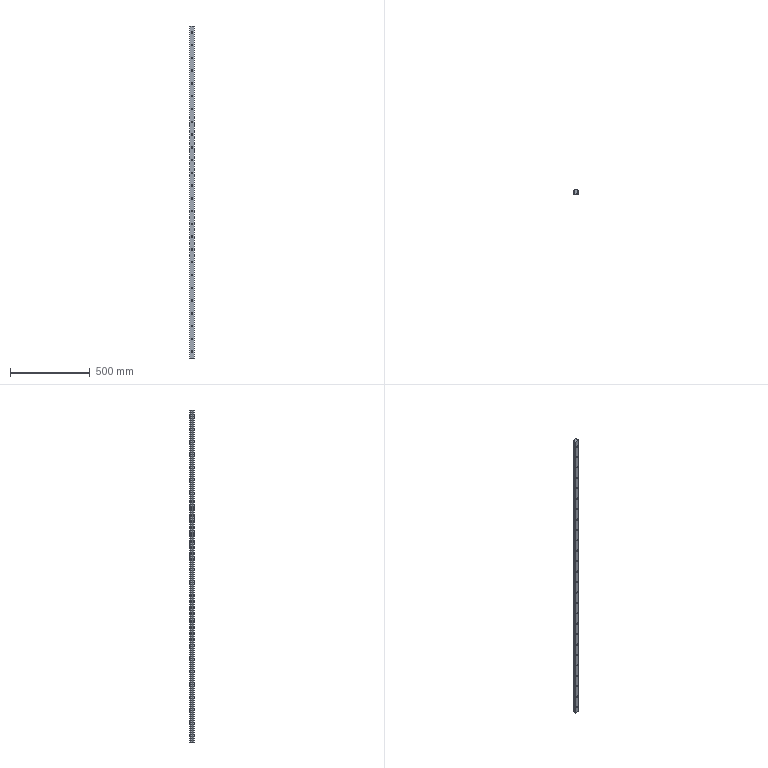Part | SolidWorks | features ICE 19, MirrorPattern 5, Extrusion 4, MirrorSolid 4, Chamfer 3, Fillet 3, RevCut 3, Dome 2, LPattern 2, DeleteBody 1, LibraryFeature 1, Revolution 1 | 1 solid | 156 faces | box 28 x 26 x 2080 mm | volume 1265174 mm3 | cylinder 110 | plane 46 | commonest cylinder face diameters 9 x52 14 x52 2.822 x6